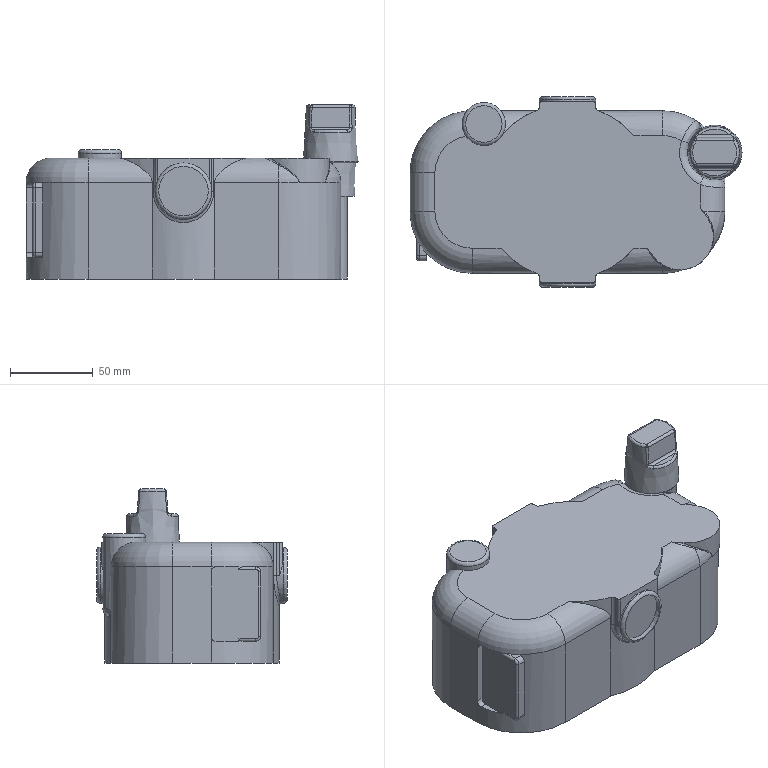Part | STEP file | Upper_shell_sub | 1 solid | 122 faces | box 200.312 x 115 x 105 mm | volume 1313356 mm3 | cylinder 41 | plane 34 | spline 22 | torus 18 | sphere 4 | cone 3 | commonest cylinder face diameters 3 x12 30 x8 75 x6 4 x4 6 x4 34 x2